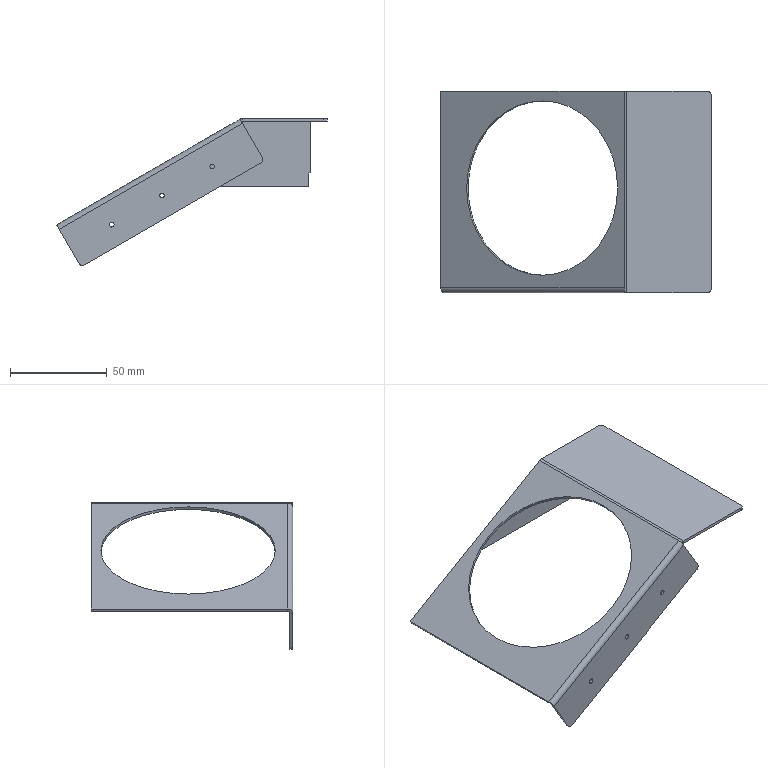Part | SolidWorks | features Cut 2, EdgeFlange 2, Fillet 1, FlatPattern 1, HoleWzd 1, ICE 1, SMBaseFlange 1, SheetMetal 1 | 1 solid | 38 faces | box 139.665 x 104 x 75.919 mm | volume 19261 mm3 | plane 22 | cylinder 16 | commonest cylinder face diameters 2.5 x6 4 x4 2 x2 5 x2 90 x2
STEP:
#1=CARTESIAN_POINT('',(-35.843,-50.5,-23.542));
#2=VERTEX_POINT('',#1);
#3=CARTESIAN_POINT('',(-35.843,-50.5,-26.042));
#4=VERTEX_POINT('',#3);
#5=CARTESIAN_POINT('',(-35.843,-50.5,-24.792));
#6=DIRECTION('',(0.,-1.,0.));
#7=DIRECTION('',(0.,0.,-1.));
#8=AXIS2_PLACEMENT_3D('',#5,#6,#7);
#9=CIRCLE('',#8,1.25);
#10=EDGE_CURVE('',#2,#4,#9,.T.);
#11=ORIENTED_EDGE('',*,*,#10,.F.);
#12=CARTESIAN_POINT('',(-35.843,-52.,-23.542));
#13=VERTEX_POINT('',#12);
#14=CARTESIAN_POINT('',(-35.843,-52.,-23.542));
#15=DIRECTION('',(0.,-1.,0.));
#16=VECTOR('',#15,1000.);
#17=LINE('',#14,#16);
#18=EDGE_CURVE('',#2,#13,#17,.T.);
#19=ORIENTED_EDGE('',*,*,#18,.T.);
#20=CARTESIAN_POINT('',(-35.843,-52.,-26.042));
#21=VERTEX_POINT('',#20);
#22=CARTESIAN_POINT('',(-35.843,-52.,-24.792));
#23=DIRECTION('',(0.,-1.,0.));
#24=DIRECTION('',(0.,0.,-1.));
#25=AXIS2_PLACEMENT_3D('',#22,#23,#24);
#26=CIRCLE('',#25,1.25);
#27=EDGE_CURVE('',#13,#21,#26,.T.);
#28=ORIENTED_EDGE('',*,*,#27,.T.);
#29=CARTESIAN_POINT('',(-35.843,-52.,-26.042));
#30=DIRECTION('',(0.,-1.,0.));
#31=VECTOR('',#30,1000.);
#32=LINE('',#29,#31);
#33=EDGE_CURVE('',#4,#21,#32,.T.);
#34=ORIENTED_EDGE('',*,*,#33,.F.);
#35=EDGE_LOOP('',(#11,#19,#28,#34));
#36=FACE_OUTER_BOUND('',#35,.T.);
#37=CARTESIAN_POINT('',(-35.843,-52.,-24.792));
#38=DIRECTION('',(0.,-1.,0.));
#39=DIRECTION('',(0.,0.,-1.));
#40=AXIS2_PLACEMENT_3D('',#37,#38,#39);
#41=CYLINDRICAL_SURFACE('',#40,1.25);
#42=ADVANCED_FACE('',(#36),#41,.F.);
#43=CARTESIAN_POINT('',(-61.823,-50.5,-38.542));
#44=VERTEX_POINT('',#43);
#45=CARTESIAN_POINT('',(-61.823,-50.5,-41.042));
#46=VERTEX_POINT('',#45);
#47=CARTESIAN_POINT('',(-61.823,-50.5,-39.792));
#48=DIRECTION('',(0.,-1.,0.));
#49=DIRECTION('',(0.,0.,-1.));
#50=AXIS2_PLACEMENT_3D('',#47,#48,#49);
#51=CIRCLE('',#50,1.25);
#52=EDGE_CURVE('',#44,#46,#51,.T.);
#53=ORIENTED_EDGE('',*,*,#52,.F.);
#54=CARTESIAN_POINT('',(-61.823,-52.,-38.542));
#55=VERTEX_POINT('',#54);
#56=CARTESIAN_POINT('',(-61.823,-52.,-38.542));
#57=DIRECTION('',(0.,-1.,0.));
#58=VECTOR('',#57,1000.);
#59=LINE('',#56,#58);
#60=EDGE_CURVE('',#44,#55,#59,.T.);
#61=ORIENTED_EDGE('',*,*,#60,.T.);
#62=CARTESIAN_POINT('',(-61.823,-52.,-41.042));
#63=VERTEX_POINT('',#62);
#64=CARTESIAN_POINT('',(-61.823,-52.,-39.792));
#65=DIRECTION('',(0.,-1.,0.));
#66=DIRECTION('',(0.,0.,-1.));
#67=AXIS2_PLACEMENT_3D('',#64,#65,#66);
#68=CIRCLE('',#67,1.25);
#69=EDGE_CURVE('',#55,#63,#68,.T.);
#70=ORIENTED_EDGE('',*,*,#69,.T.);
#71=CARTESIAN_POINT('',(-61.823,-52.,-41.042));
#72=DIRECTION('',(0.,-1.,0.));
#73=VECTOR('',#72,1000.);
#74=LINE('',#71,#73);
#75=EDGE_CURVE('',#46,#63,#74,.T.);
#76=ORIENTED_EDGE('',*,*,#75,.F.);
#77=EDGE_LOOP('',(#53,#61,#70,#76));
#78=FACE_OUTER_BOUND('',#77,.T.);
#79=CARTESIAN_POINT('',(-61.823,-52.,-39.792));
#80=DIRECTION('',(0.,-1.,0.));
#81=DIRECTION('',(0.,0.,-1.));
#82=AXIS2_PLACEMENT_3D('',#79,#80,#81);
#83=CYLINDRICAL_SURFACE('',#82,1.25);
#84=ADVANCED_FACE('',(#78),#83,.F.);
#85=CARTESIAN_POINT('',(-87.804,-50.5,-53.542));
#86=VERTEX_POINT('',#85);
#87=CARTESIAN_POINT('',(-87.804,-50.5,-56.042));
#88=VERTEX_POINT('',#87);
#89=CARTESIAN_POINT('',(-87.804,-50.5,-54.792));
#90=DIRECTION('',(0.,-1.,0.));
#91=DIRECTION('',(0.,0.,-1.));
#92=AXIS2_PLACEMENT_3D('',#89,#90,#91);
#93=CIRCLE('',#92,1.25);
#94=EDGE_CURVE('',#86,#88,#93,.T.);
#95=ORIENTED_EDGE('',*,*,#94,.F.);
#96=CARTESIAN_POINT('',(-87.804,-52.,-53.542));
#97=VERTEX_POINT('',#96);
#98=CARTESIAN_POINT('',(-87.804,-52.,-53.542));
#99=DIRECTION('',(0.,-1.,0.));
#100=VECTOR('',#99,1000.);
#101=LINE('',#98,#100);
#102=EDGE_CURVE('',#86,#97,#101,.T.);
#103=ORIENTED_EDGE('',*,*,#102,.T.);
#104=CARTESIAN_POINT('',(-87.804,-52.,-56.042));
#105=VERTEX_POINT('',#104);
#106=CARTESIAN_POINT('',(-87.804,-52.,-54.792));
#107=DIRECTION('',(0.,-1.,0.));
#108=DIRECTION('',(0.,0.,-1.));
#109=AXIS2_PLACEMENT_3D('',#106,#107,#108);
#110=CIRCLE('',#109,1.25);
#111=EDGE_CURVE('',#97,#105,#110,.T.);
#112=ORIENTED_EDGE('',*,*,#111,.T.);
#113=CARTESIAN_POINT('',(-87.804,-52.,-56.042));
#114=DIRECTION('',(0.,-1.,0.));
#115=VECTOR('',#114,1000.);
#116=LINE('',#113,#115);
#117=EDGE_CURVE('',#88,#105,#116,.T.);
#118=ORIENTED_EDGE('',*,*,#117,.F.);
#119=EDGE_LOOP('',(#95,#103,#112,#118));
#120=FACE_OUTER_BOUND('',#119,.T.);
#121=CARTESIAN_POINT('',(-87.804,-52.,-54.792));
#122=DIRECTION('',(0.,-1.,0.));
#123=DIRECTION('',(0.,0.,-1.));
#124=AXIS2_PLACEMENT_3D('',#121,#122,#123);
#125=CYLINDRICAL_SURFACE('',#124,1.25);
#126=ADVANCED_FACE('',(#120),#125,.F.);
#127=CARTESIAN_POINT('',(-102.041,2.,-48.578));
#128=VERTEX_POINT('',#127);
#129=CARTESIAN_POINT('',(-24.099,2.,-3.578));
#130=VERTEX_POINT('',#129);
#131=CARTESIAN_POINT('',(-63.07,2.,-26.078));
#132=DIRECTION('',(-0.5,0.,0.866));
#133=DIRECTION('',(0.866,0.,0.5));
#134=AXIS2_PLACEMENT_3D('',#131,#132,#133);
#135=CIRCLE('',#134,45.);
#136=EDGE_CURVE('',#128,#130,#135,.T.);
#137=ORIENTED_EDGE('',*,*,#136,.F.);
#138=CARTESIAN_POINT('',(-102.791,2.,-47.279));
#139=VERTEX_POINT('',#138);
#140=CARTESIAN_POINT('',(-97.791,2.,-55.939));
#141=DIRECTION('',(-0.5,0.,0.866));
#142=VECTOR('',#141,1000.);
#143=LINE('',#140,#142);
#144=EDGE_CURVE('',#128,#139,#143,.T.);
#145=ORIENTED_EDGE('',*,*,#144,.T.);
#146=CARTESIAN_POINT('',(-24.849,2.,-2.279));
#147=VERTEX_POINT('',#146);
#148=CARTESIAN_POINT('',(-63.82,2.,-24.779));
#149=DIRECTION('',(-0.5,0.,0.866));
#150=DIRECTION('',(0.866,0.,0.5));
#151=AXIS2_PLACEMENT_3D('',#148,#149,#150);
#152=CIRCLE('',#151,45.);
#153=EDGE_CURVE('',#139,#147,#152,.T.);
#154=ORIENTED_EDGE('',*,*,#153,.T.);
#155=CARTESIAN_POINT('',(-19.849,2.,-10.939));
#156=DIRECTION('',(-0.5,0.,0.866));
#157=VECTOR('',#156,1000.);
#158=LINE('',#155,#157);
#159=EDGE_CURVE('',#130,#147,#158,.T.);
#160=ORIENTED_EDGE('',*,*,#159,.F.);
#161=EDGE_LOOP('',(#137,#145,#154,#160));
#162=FACE_OUTER_BOUND('',#161,.T.);
#163=CARTESIAN_POINT('',(-58.82,2.,-33.439));
#164=DIRECTION('',(-0.5,0.,0.866));
#165=DIRECTION('',(0.866,0.,0.5));
#166=AXIS2_PLACEMENT_3D('',#163,#164,#165);
#167=CYLINDRICAL_SURFACE('',#166,45.);
#168=ADVANCED_FACE('',(#162),#167,.F.);
#169=CARTESIAN_POINT('',(-20.732,51.5,-1.634));
#170=VERTEX_POINT('',#169);
#171=CARTESIAN_POINT('',(-20.232,51.5,-1.5));
#172=VERTEX_POINT('',#171);
#173=CARTESIAN_POINT('',(-20.232,51.5,-2.5));
#174=DIRECTION('',(0.,1.,0.));
#175=DIRECTION('',(0.,0.,1.));
#176=AXIS2_PLACEMENT_3D('',#173,#174,#175);
#177=CIRCLE('',#176,1.);
#178=EDGE_CURVE('',#170,#172,#177,.T.);
#179=ORIENTED_EDGE('',*,*,#178,.T.);
#180=CARTESIAN_POINT('',(-20.232,-52.,-1.5));
#181=VERTEX_POINT('',#180);
#182=CARTESIAN_POINT('',(-20.232,52.,-1.5));
#183=DIRECTION('',(0.,-1.,0.));
#184=VECTOR('',#183,1000.);
#185=LINE('',#182,#184);
#186=EDGE_CURVE('',#172,#181,#185,.T.);
#187=ORIENTED_EDGE('',*,*,#186,.T.);
#188=CARTESIAN_POINT('',(-20.732,-52.,-1.634));
#189=VERTEX_POINT('',#188);
#190=CARTESIAN_POINT('',(-20.232,-52.,-2.5));
#191=DIRECTION('',(0.,-1.,0.));
#192=DIRECTION('',(0.,0.,1.));
#193=AXIS2_PLACEMENT_3D('',#190,#191,#192);
#194=CIRCLE('',#193,1.);
#195=EDGE_CURVE('',#181,#189,#194,.T.);
#196=ORIENTED_EDGE('',*,*,#195,.T.);
#197=CARTESIAN_POINT('',(-20.732,-51.791,-1.634));
#198=VERTEX_POINT('',#197);
#199=CARTESIAN_POINT('',(-20.732,-52.,-1.634));
#200=DIRECTION('',(0.,1.,0.));
#201=VECTOR('',#200,1000.);
#202=LINE('',#199,#201);
#203=EDGE_CURVE('',#189,#198,#202,.T.);
#204=ORIENTED_EDGE('',*,*,#203,.T.);
#205=CARTESIAN_POINT('',(-20.732,-49.5,-1.634));
#206=VERTEX_POINT('',#205);
#207=CARTESIAN_POINT('',(-20.732,-52.,-1.634));
#208=DIRECTION('',(0.,1.,0.));
#209=VECTOR('',#208,1000.);
#210=LINE('',#207,#209);
#211=EDGE_CURVE('',#198,#206,#210,.T.);
#212=ORIENTED_EDGE('',*,*,#211,.T.);
#213=CARTESIAN_POINT('',(-20.732,-52.,-1.634));
#214=DIRECTION('',(0.,1.,0.));
#215=VECTOR('',#214,1000.);
#216=LINE('',#213,#215);
#217=EDGE_CURVE('',#206,#170,#216,.T.);
#218=ORIENTED_EDGE('',*,*,#217,.T.);
#219=EDGE_LOOP('',(#179,#187,#196,#204,#212,#218));
#220=FACE_OUTER_BOUND('',#219,.T.);
#221=CARTESIAN_POINT('',(-20.232,52.,-2.5));
#222=DIRECTION('',(0.,1.,0.));
#223=DIRECTION('',(-0.5,0.,0.866));
#224=AXIS2_PLACEMENT_3D('',#221,#222,#223);
#225=CYLINDRICAL_SURFACE('',#224,1.);
#226=ADVANCED_FACE('',(#220),#225,.F.);
#227=CARTESIAN_POINT('',(-21.482,-52.,-0.3349));
#228=VERTEX_POINT('',#227);
#229=CARTESIAN_POINT('',(-21.482,-49.5,-0.3349));
#230=VERTEX_POINT('',#229);
#231=CARTESIAN_POINT('',(-21.482,0.,-0.3349));
#232=DIRECTION('',(0.,1.,0.));
#233=VECTOR('',#232,1000.);
#234=LINE('',#231,#233);
#235=EDGE_CURVE('',#228,#230,#234,.T.);
#236=ORIENTED_EDGE('',*,*,#235,.T.);
#237=CARTESIAN_POINT('',(-20.232,-49.5,-2.5));
#238=DIRECTION('',(0.866,0.,0.5));
#239=DIRECTION('',(-0.5,0.,0.866));
#240=AXIS2_PLACEMENT_3D('',#237,#238,#239);
#241=CIRCLE('',#240,2.5);
#242=EDGE_CURVE('',#230,#198,#241,.T.);
#243=ORIENTED_EDGE('',*,*,#242,.T.);
#244=ORIENTED_EDGE('',*,*,#203,.F.);
#245=CARTESIAN_POINT('',(-21.482,-52.,-0.3349));
#246=DIRECTION('',(-0.5,0.,0.866));
#247=VECTOR('',#246,1000.);
#248=LINE('',#245,#247);
#249=EDGE_CURVE('',#189,#228,#248,.T.);
#250=ORIENTED_EDGE('',*,*,#249,.T.);
#251=EDGE_LOOP('',(#236,#243,#244,#250));
#252=FACE_OUTER_BOUND('',#251,.T.);
#253=CARTESIAN_POINT('',(-20.732,-49.5,-1.634));
#254=DIRECTION('',(-0.866,0.,-0.5));
#255=DIRECTION('',(-0.5,0.,0.866));
#256=AXIS2_PLACEMENT_3D('',#253,#254,#255);
#257=PLANE('',#256);
#258=ADVANCED_FACE('',(#252),#257,.T.);
#259=CARTESIAN_POINT('',(-63.82,2.,-24.779));
#260=DIRECTION('',(-0.5,0.,0.866));
#261=DIRECTION('',(0.866,0.,0.5));
#262=AXIS2_PLACEMENT_3D('',#259,#260,#261);
#263=CIRCLE('',#262,45.);
#264=EDGE_CURVE('',#147,#139,#263,.T.);
#265=ORIENTED_EDGE('',*,*,#264,.F.);
#266=ORIENTED_EDGE('',*,*,#153,.F.);
#267=EDGE_LOOP('',(#265,#266));
#268=FACE_BOUND('',#267,.T.);
#269=CARTESIAN_POINT('',(-116.165,-49.5,-55.));
#270=VERTEX_POINT('',#269);
#271=CARTESIAN_POINT('',(-116.165,52.,-55.));
#272=VERTEX_POINT('',#271);
#273=CARTESIAN_POINT('',(-116.165,52.,-55.));
#274=DIRECTION('',(0.,1.,0.));
#275=VECTOR('',#274,1000.);
#276=LINE('',#273,#275);
#277=EDGE_CURVE('',#270,#272,#276,.T.);
#278=ORIENTED_EDGE('',*,*,#277,.F.);
#279=CARTESIAN_POINT('',(-116.165,-49.5,-55.));
#280=DIRECTION('',(0.866,0.,0.5));
#281=VECTOR('',#280,1000.);
#282=LINE('',#279,#281);
#283=EDGE_CURVE('',#270,#230,#282,.T.);
#284=ORIENTED_EDGE('',*,*,#283,.T.);
#285=CARTESIAN_POINT('',(-21.482,52.,-0.3349));
#286=VERTEX_POINT('',#285);
#287=CARTESIAN_POINT('',(-21.482,0.,-0.3349));
#288=DIRECTION('',(0.,1.,0.));
#289=VECTOR('',#288,1000.);
#290=LINE('',#287,#289);
#291=EDGE_CURVE('',#230,#286,#290,.T.);
#292=ORIENTED_EDGE('',*,*,#291,.T.);
#293=CARTESIAN_POINT('',(-21.25,52.,-0.201));
#294=DIRECTION('',(0.866,0.,0.5));
#295=VECTOR('',#294,1000.);
#296=LINE('',#293,#295);
#297=EDGE_CURVE('',#272,#286,#296,.T.);
#298=ORIENTED_EDGE('',*,*,#297,.F.);
#299=EDGE_LOOP('',(#278,#284,#292,#298));
#300=FACE_OUTER_BOUND('',#299,.T.);
#301=CARTESIAN_POINT('',(-2.975,0.,10.35));
#302=DIRECTION('',(-0.5,0.,0.866));
#303=DIRECTION('',(0.866,0.,0.5));
#304=AXIS2_PLACEMENT_3D('',#301,#302,#303);
#305=PLANE('',#304);
#306=ADVANCED_FACE('',(#268,#300),#305,.T.);
#307=CARTESIAN_POINT('',(-63.07,2.,-26.078));
#308=DIRECTION('',(-0.5,0.,0.866));
#309=DIRECTION('',(0.866,0.,0.5));
#310=AXIS2_PLACEMENT_3D('',#307,#308,#309);
#311=CIRCLE('',#310,45.);
#312=EDGE_CURVE('',#130,#128,#311,.T.);
#313=ORIENTED_EDGE('',*,*,#312,.T.);
#314=ORIENTED_EDGE('',*,*,#136,.T.);
#315=EDGE_LOOP('',(#313,#314));
#316=FACE_BOUND('',#315,.T.);
#317=CARTESIAN_POINT('',(-115.415,52.,-56.299));
#318=VERTEX_POINT('',#317);
#319=CARTESIAN_POINT('',(-78.756,52.,-35.134));
#320=VERTEX_POINT('',#319);
#321=CARTESIAN_POINT('',(-2.225,52.,9.051));
#322=DIRECTION('',(0.866,0.,0.5));
#323=VECTOR('',#322,1000.);
#324=LINE('',#321,#323);
#325=EDGE_CURVE('',#318,#320,#324,.T.);
#326=ORIENTED_EDGE('',*,*,#325,.T.);
#327=CARTESIAN_POINT('',(-78.756,51.5,-35.134));
#328=VERTEX_POINT('',#327);
#329=CARTESIAN_POINT('',(-78.756,51.5,-35.134));
#330=DIRECTION('',(0.,1.,0.));
#331=VECTOR('',#330,1000.);
#332=LINE('',#329,#331);
#333=EDGE_CURVE('',#328,#320,#332,.T.);
#334=ORIENTED_EDGE('',*,*,#333,.F.);
#335=CARTESIAN_POINT('',(-20.732,51.5,-1.634));
#336=DIRECTION('',(0.866,0.,0.5));
#337=VECTOR('',#336,1000.);
#338=LINE('',#335,#337);
#339=EDGE_CURVE('',#328,#170,#338,.T.);
#340=ORIENTED_EDGE('',*,*,#339,.T.);
#341=ORIENTED_EDGE('',*,*,#217,.F.);
#342=CARTESIAN_POINT('',(-115.415,-49.5,-56.299));
#343=VERTEX_POINT('',#342);
#344=CARTESIAN_POINT('',(-115.415,-49.5,-56.299));
#345=DIRECTION('',(0.866,0.,0.5));
#346=VECTOR('',#345,1000.);
#347=LINE('',#344,#346);
#348=EDGE_CURVE('',#343,#206,#347,.T.);
#349=ORIENTED_EDGE('',*,*,#348,.F.);
#350=CARTESIAN_POINT('',(-115.415,0.,-56.299));
#351=DIRECTION('',(0.,1.,0.));
#352=VECTOR('',#351,1000.);
#353=LINE('',#350,#352);
#354=EDGE_CURVE('',#343,#318,#353,.T.);
#355=ORIENTED_EDGE('',*,*,#354,.T.);
#356=EDGE_LOOP('',(#326,#334,#340,#341,#349,#355));
#357=FACE_OUTER_BOUND('',#356,.T.);
#358=CARTESIAN_POINT('',(-2.225,0.,9.051));
#359=DIRECTION('',(-0.5,0.,0.866));
#360=DIRECTION('',(0.866,0.,0.5));
#361=AXIS2_PLACEMENT_3D('',#358,#359,#360);
#362=PLANE('',#361);
#363=ADVANCED_FACE('',(#316,#357),#362,.F.);
#364=ORIENTED_EDGE('',*,*,#354,.F.);
#365=CARTESIAN_POINT('',(-115.415,-49.5,-56.299));
#366=DIRECTION('',(-0.5,0.,0.866));
#367=VECTOR('',#366,1000.);
#368=LINE('',#365,#367);
#369=EDGE_CURVE('',#343,#270,#368,.T.);
#370=ORIENTED_EDGE('',*,*,#369,.T.);
#371=ORIENTED_EDGE('',*,*,#277,.T.);
#372=CARTESIAN_POINT('',(-116.165,52.,-55.));
#373=DIRECTION('',(0.5,0.,-0.866));
#374=VECTOR('',#373,1000.);
#375=LINE('',#372,#374);
#376=EDGE_CURVE('',#272,#318,#375,.T.);
#377=ORIENTED_EDGE('',*,*,#376,.T.);
#378=EDGE_LOOP('',(#364,#370,#371,#377));
#379=FACE_OUTER_BOUND('',#378,.T.);
#380=CARTESIAN_POINT('',(-116.165,52.,-55.));
#381=DIRECTION('',(-0.866,0.,-0.5));
#382=DIRECTION('',(-0.5,0.,0.866));
#383=AXIS2_PLACEMENT_3D('',#380,#381,#382);
#384=PLANE('',#383);
#385=ADVANCED_FACE('',(#379),#384,.T.);
#386=CARTESIAN_POINT('',(-20.232,52.,0.));
#387=VERTEX_POINT('',#386);
#388=CARTESIAN_POINT('',(-20.232,52.,-2.5));
#389=DIRECTION('',(0.,1.,0.));
#390=DIRECTION('',(0.,0.,1.));
#391=AXIS2_PLACEMENT_3D('',#388,#389,#390);
#392=CIRCLE('',#391,2.5);
#393=EDGE_CURVE('',#286,#387,#392,.T.);
#394=ORIENTED_EDGE('',*,*,#393,.T.);
#395=CARTESIAN_POINT('',(21.5,52.,0.));
#396=VERTEX_POINT('',#395);
#397=CARTESIAN_POINT('',(-23.5,52.,0.));
#398=DIRECTION('',(-1.,0.,0.));
#399=VECTOR('',#398,1000.);
#400=LINE('',#397,#399);
#401=EDGE_CURVE('',#396,#387,#400,.T.);
#402=ORIENTED_EDGE('',*,*,#401,.F.);
#403=CARTESIAN_POINT('',(21.5,52.,-1.5));
#404=VERTEX_POINT('',#403);
#405=CARTESIAN_POINT('',(21.5,52.,-1.5));
#406=DIRECTION('',(0.,0.,-1.));
#407=VECTOR('',#406,1000.);
#408=LINE('',#405,#407);
#409=EDGE_CURVE('',#396,#404,#408,.T.);
#410=ORIENTED_EDGE('',*,*,#409,.T.);
#411=CARTESIAN_POINT('',(14.768,52.,-1.5));
#412=VERTEX_POINT('',#411);
#413=CARTESIAN_POINT('',(-23.5,52.,-1.5));
#414=DIRECTION('',(-1.,0.,0.));
#415=VECTOR('',#414,1000.);
#416=LINE('',#413,#415);
#417=EDGE_CURVE('',#404,#412,#416,.T.);
#418=ORIENTED_EDGE('',*,*,#417,.T.);
#419=CARTESIAN_POINT('',(14.768,52.,-28.134));
#420=VERTEX_POINT('',#419);
#421=CARTESIAN_POINT('',(14.768,52.,-1.5));
#422=DIRECTION('',(0.,0.,-1.));
#423=VECTOR('',#422,1000.);
#424=LINE('',#421,#423);
#425=EDGE_CURVE('',#412,#420,#424,.T.);
#426=ORIENTED_EDGE('',*,*,#425,.T.);
#427=CARTESIAN_POINT('',(13.843,52.,-28.134));
#428=VERTEX_POINT('',#427);
#429=CARTESIAN_POINT('',(14.768,52.,-28.134));
#430=DIRECTION('',(1.,0.,0.));
#431=VECTOR('',#430,1000.);
#432=LINE('',#429,#431);
#433=EDGE_CURVE('',#428,#420,#432,.T.);
#434=ORIENTED_EDGE('',*,*,#433,.F.);
#435=CARTESIAN_POINT('',(13.843,52.,-35.134));
#436=VERTEX_POINT('',#435);
#437=CARTESIAN_POINT('',(13.843,52.,-35.134));
#438=DIRECTION('',(0.,0.,1.));
#439=VECTOR('',#438,1000.);
#440=LINE('',#437,#439);
#441=EDGE_CURVE('',#436,#428,#440,.T.);
#442=ORIENTED_EDGE('',*,*,#441,.F.);
#443=CARTESIAN_POINT('',(14.768,52.,-35.134));
#444=DIRECTION('',(-1.,0.,0.));
#445=VECTOR('',#444,1000.);
#446=LINE('',#443,#445);
#447=EDGE_CURVE('',#436,#320,#446,.T.);
#448=ORIENTED_EDGE('',*,*,#447,.T.);
#449=ORIENTED_EDGE('',*,*,#325,.F.);
#450=ORIENTED_EDGE('',*,*,#376,.F.);
#451=ORIENTED_EDGE('',*,*,#297,.T.);
#452=EDGE_LOOP('',(#394,#402,#410,#418,#426,#434,#442,#448,#449,#450,#451));
#453=FACE_OUTER_BOUND('',#452,.T.);
#454=CARTESIAN_POINT('',(-23.5,52.,-1.5));
#455=DIRECTION('',(0.,1.,0.));
#456=DIRECTION('',(0.,0.,1.));
#457=AXIS2_PLACEMENT_3D('',#454,#455,#456);
#458=PLANE('',#457);
#459=ADVANCED_FACE('',(#453),#458,.T.);
#460=CARTESIAN_POINT('',(14.768,51.5,-1.5));
#461=VERTEX_POINT('',#460);
#462=CARTESIAN_POINT('',(-20.232,51.5,-1.5));
#463=DIRECTION('',(1.,0.,0.));
#464=VECTOR('',#463,1000.);
#465=LINE('',#462,#464);
#466=EDGE_CURVE('',#172,#461,#465,.T.);
#467=ORIENTED_EDGE('',*,*,#466,.T.);
#468=CARTESIAN_POINT('',(14.768,51.5,-1.5));
#469=DIRECTION('',(0.,1.,0.));
#470=VECTOR('',#469,1000.);
#471=LINE('',#468,#470);
#472=EDGE_CURVE('',#461,#412,#471,.T.);
#473=ORIENTED_EDGE('',*,*,#472,.T.);
#474=ORIENTED_EDGE('',*,*,#417,.F.);
#475=CARTESIAN_POINT('',(23.5,50.,-1.5));
#476=VERTEX_POINT('',#475);
#477=CARTESIAN_POINT('',(21.5,50.,-1.5));
#478=DIRECTION('',(0.,0.,-1.));
#479=DIRECTION('',(1.,0.,0.));
#480=AXIS2_PLACEMENT_3D('',#477,#478,#479);
#481=CIRCLE('',#480,2.);
#482=EDGE_CURVE('',#404,#476,#481,.T.);
#483=ORIENTED_EDGE('',*,*,#482,.T.);
#484=CARTESIAN_POINT('',(23.5,-50.,-1.5));
#485=VERTEX_POINT('',#484);
#486=CARTESIAN_POINT('',(23.5,52.,-1.5));
#487=DIRECTION('',(0.,1.,0.));
#488=VECTOR('',#487,1000.);
#489=LINE('',#486,#488);
#490=EDGE_CURVE('',#485,#476,#489,.T.);
#491=ORIENTED_EDGE('',*,*,#490,.F.);
#492=CARTESIAN_POINT('',(21.5,-52.,-1.5));
#493=VERTEX_POINT('',#492);
#494=CARTESIAN_POINT('',(21.5,-50.,-1.5));
#495=DIRECTION('',(0.,0.,-1.));
#496=DIRECTION('',(1.,0.,0.));
#497=AXIS2_PLACEMENT_3D('',#494,#495,#496);
#498=CIRCLE('',#497,2.);
#499=EDGE_CURVE('',#485,#493,#498,.T.);
#500=ORIENTED_EDGE('',*,*,#499,.T.);
#501=CARTESIAN_POINT('',(-23.5,-52.,-1.5));
#502=DIRECTION('',(1.,0.,0.));
#503=VECTOR('',#502,1000.);
#504=LINE('',#501,#503);
#505=EDGE_CURVE('',#181,#493,#504,.T.);
#506=ORIENTED_EDGE('',*,*,#505,.F.);
#507=ORIENTED_EDGE('',*,*,#186,.F.);
#508=EDGE_LOOP('',(#467,#473,#474,#483,#491,#500,#506,#507));
#509=FACE_OUTER_BOUND('',#508,.T.);
#510=CARTESIAN_POINT('',(0.,0.,-1.5));
#511=DIRECTION('',(0.,0.,1.));
#512=DIRECTION('',(1.,0.,0.));
#513=AXIS2_PLACEMENT_3D('',#510,#511,#512);
#514=PLANE('',#513);
#515=ADVANCED_FACE('',(#509),#514,.F.);
#516=CARTESIAN_POINT('',(23.5,-50.,0.));
#517=VERTEX_POINT('',#516);
#518=CARTESIAN_POINT('',(23.5,50.,0.));
#519=VERTEX_POINT('',#518);
#520=CARTESIAN_POINT('',(23.5,52.,0.));
#521=DIRECTION('',(0.,1.,0.));
#522=VECTOR('',#521,1000.);
#523=LINE('',#520,#522);
#524=EDGE_CURVE('',#517,#519,#523,.T.);
#525=ORIENTED_EDGE('',*,*,#524,.T.);
#526=CARTESIAN_POINT('',(21.5,50.,0.));
#527=DIRECTION('',(0.,0.,1.));
#528=DIRECTION('',(1.,0.,0.));
#529=AXIS2_PLACEMENT_3D('',#526,#527,#528);
#530=CIRCLE('',#529,2.);
#531=EDGE_CURVE('',#519,#396,#530,.T.);
#532=ORIENTED_EDGE('',*,*,#531,.T.);
#533=ORIENTED_EDGE('',*,*,#401,.T.);
#534=CARTESIAN_POINT('',(-20.232,-52.,0.));
#535=VERTEX_POINT('',#534);
#536=CARTESIAN_POINT('',(-20.232,52.,0.));
#537=DIRECTION('',(0.,-1.,0.));
#538=VECTOR('',#537,1000.);
#539=LINE('',#536,#538);
#540=EDGE_CURVE('',#387,#535,#539,.T.);
#541=ORIENTED_EDGE('',*,*,#540,.T.);
#542=CARTESIAN_POINT('',(21.5,-52.,0.));
#543=VERTEX_POINT('',#542);
#544=CARTESIAN_POINT('',(-23.5,-52.,0.));
#545=DIRECTION('',(1.,0.,0.));
#546=VECTOR('',#545,1000.);
#547=LINE('',#544,#546);
#548=EDGE_CURVE('',#535,#543,#547,.T.);
#549=ORIENTED_EDGE('',*,*,#548,.T.);
#550=CARTESIAN_POINT('',(21.5,-50.,0.));
#551=DIRECTION('',(0.,0.,1.));
#552=DIRECTION('',(1.,0.,0.));
#553=AXIS2_PLACEMENT_3D('',#550,#551,#552);
#554=CIRCLE('',#553,2.);
#555=EDGE_CURVE('',#543,#517,#554,.T.);
#556=ORIENTED_EDGE('',*,*,#555,.T.);
#557=EDGE_LOOP('',(#525,#532,#533,#541,#549,#556));
#558=FACE_OUTER_BOUND('',#557,.T.);
#559=CARTESIAN_POINT('',(0.,0.,0.));
#560=DIRECTION('',(0.,0.,1.));
#561=DIRECTION('',(1.,0.,0.));
#562=AXIS2_PLACEMENT_3D('',#559,#560,#561);
#563=PLANE('',#562);
#564=ADVANCED_FACE('',(#558),#563,.T.);
#565=ORIENTED_EDGE('',*,*,#490,.T.);
#566=CARTESIAN_POINT('',(23.5,50.,-1.5));
#567=DIRECTION('',(0.,0.,1.));
#568=VECTOR('',#567,1000.);
#569=LINE('',#566,#568);
#570=EDGE_CURVE('',#476,#519,#569,.T.);
#571=ORIENTED_EDGE('',*,*,#570,.T.);
#572=ORIENTED_EDGE('',*,*,#524,.F.);
#573=CARTESIAN_POINT('',(23.5,-50.,-1.5));
#574=DIRECTION('',(0.,0.,-1.));
#575=VECTOR('',#574,1000.);
#576=LINE('',#573,#575);
#577=EDGE_CURVE('',#517,#485,#576,.T.);
#578=ORIENTED_EDGE('',*,*,#577,.T.);
#579=EDGE_LOOP('',(#565,#571,#572,#578));
#580=FACE_OUTER_BOUND('',#579,.T.);
#581=CARTESIAN_POINT('',(23.5,52.,-1.5));
#582=DIRECTION('',(1.,0.,0.));
#583=DIRECTION('',(0.,1.,0.));
#584=AXIS2_PLACEMENT_3D('',#581,#582,#583);
#585=PLANE('',#584);
#586=ADVANCED_FACE('',(#580),#585,.T.);
#587=ORIENTED_EDGE('',*,*,#505,.T.);
#588=CARTESIAN_POINT('',(21.5,-52.,-1.5));
#589=DIRECTION('',(0.,0.,1.));
#590=VECTOR('',#589,1000.);
#591=LINE('',#588,#590);
#592=EDGE_CURVE('',#493,#543,#591,.T.);
#593=ORIENTED_EDGE('',*,*,#592,.T.);
#594=ORIENTED_EDGE('',*,*,#548,.F.);
#595=CARTESIAN_POINT('',(-20.232,-52.,-1.5));
#596=DIRECTION('',(0.,0.,1.));
#597=VECTOR('',#596,1000.);
#598=LINE('',#595,#597);
#599=EDGE_CURVE('',#181,#535,#598,.T.);
#600=ORIENTED_EDGE('',*,*,#599,.F.);
#601=EDGE_LOOP('',(#587,#593,#594,#600));
#602=FACE_OUTER_BOUND('',#601,.T.);
#603=CARTESIAN_POINT('',(-23.5,-52.,-1.5));
#604=DIRECTION('',(0.,-1.,0.));
#605=DIRECTION('',(0.,0.,-1.));
#606=AXIS2_PLACEMENT_3D('',#603,#604,#605);
#607=PLANE('',#606);
#608=ADVANCED_FACE('',(#602),#607,.T.);
#609=ORIENTED_EDGE('',*,*,#249,.F.);
#610=ORIENTED_EDGE('',*,*,#195,.F.);
#611=ORIENTED_EDGE('',*,*,#599,.T.);
#612=CARTESIAN_POINT('',(-20.232,-52.,-2.5));
#613=DIRECTION('',(0.,-1.,0.));
#614=DIRECTION('',(0.,0.,1.));
#615=AXIS2_PLACEMENT_3D('',#612,#613,#614);
#616=CIRCLE('',#615,2.5);
#617=EDGE_CURVE('',#535,#228,#616,.T.);
#618=ORIENTED_EDGE('',*,*,#617,.T.);
#619=EDGE_LOOP('',(#609,#610,#611,#618));
#620=FACE_OUTER_BOUND('',#619,.T.);
#621=CARTESIAN_POINT('',(-20.232,-52.,-2.5));
#622=DIRECTION('',(0.,-1.,0.));
#623=DIRECTION('',(0.,0.,-1.));
#624=AXIS2_PLACEMENT_3D('',#621,#622,#623);
#625=PLANE('',#624);
#626=ADVANCED_FACE('',(#620),#625,.T.);
#627=ORIENTED_EDGE('',*,*,#540,.F.);
#628=ORIENTED_EDGE('',*,*,#393,.F.);
#629=ORIENTED_EDGE('',*,*,#291,.F.);
#630=ORIENTED_EDGE('',*,*,#235,.F.);
#631=ORIENTED_EDGE('',*,*,#617,.F.);
#632=EDGE_LOOP('',(#627,#628,#629,#630,#631));
#633=FACE_OUTER_BOUND('',#632,.T.);
#634=CARTESIAN_POINT('',(-20.232,52.,-2.5));
#635=DIRECTION('',(0.,1.,0.));
#636=DIRECTION('',(-0.5,0.,0.866));
#637=AXIS2_PLACEMENT_3D('',#634,#635,#636);
#638=CYLINDRICAL_SURFACE('',#637,2.5);
#639=ADVANCED_FACE('',(#633),#638,.T.);
#640=ORIENTED_EDGE('',*,*,#211,.F.);
#641=CARTESIAN_POINT('',(-20.232,-52.,-2.5));
#642=VERTEX_POINT('',#641);
#643=CARTESIAN_POINT('',(-20.232,-49.5,-2.5));
#644=DIRECTION('',(0.866,0.,0.5));
#645=DIRECTION('',(-0.5,0.,0.866));
#646=AXIS2_PLACEMENT_3D('',#643,#644,#645);
#647=CIRCLE('',#646,2.5);
#648=EDGE_CURVE('',#198,#642,#647,.T.);
#649=ORIENTED_EDGE('',*,*,#648,.T.);
#650=CARTESIAN_POINT('',(-20.232,-50.5,-2.5));
#651=VERTEX_POINT('',#650);
#652=CARTESIAN_POINT('',(-20.232,-52.,-2.5));
#653=DIRECTION('',(0.,-1.,0.));
#654=VECTOR('',#653,1000.);
#655=LINE('',#652,#654);
#656=EDGE_CURVE('',#651,#642,#655,.T.);
#657=ORIENTED_EDGE('',*,*,#656,.F.);
#658=CARTESIAN_POINT('',(-20.232,-49.5,-2.5));
#659=DIRECTION('',(0.866,0.,0.5));
#660=DIRECTION('',(-0.5,0.,0.866));
#661=AXIS2_PLACEMENT_3D('',#658,#659,#660);
#662=CIRCLE('',#661,1.);
#663=EDGE_CURVE('',#206,#651,#662,.T.);
#664=ORIENTED_EDGE('',*,*,#663,.F.);
#665=EDGE_LOOP('',(#640,#649,#657,#664));
#666=FACE_OUTER_BOUND('',#665,.T.);
#667=CARTESIAN_POINT('',(-20.232,-49.5,-2.5));
#668=DIRECTION('',(0.866,0.,0.5));
#669=DIRECTION('',(0.5,0.,-0.866));
#670=AXIS2_PLACEMENT_3D('',#667,#668,#669);
#671=PLANE('',#670);
#672=ADVANCED_FACE('',(#666),#671,.T.);
#673=CARTESIAN_POINT('',(-114.915,-50.5,-57.165));
#674=VERTEX_POINT('',#673);
#675=CARTESIAN_POINT('',(-114.915,-49.5,-57.165));
#676=DIRECTION('',(-0.866,0.,-0.5));
#677=DIRECTION('',(-0.5,0.,0.866));
#678=AXIS2_PLACEMENT_3D('',#675,#676,#677);
#679=CIRCLE('',#678,1.);
#680=EDGE_CURVE('',#674,#343,#679,.T.);
#681=ORIENTED_EDGE('',*,*,#680,.F.);
#682=CARTESIAN_POINT('',(-114.915,-52.,-57.165));
#683=VERTEX_POINT('',#682);
#684=CARTESIAN_POINT('',(-114.915,-50.5,-57.165));
#685=DIRECTION('',(0.,-1.,0.));
#686=VECTOR('',#685,1000.);
#687=LINE('',#684,#686);
#688=EDGE_CURVE('',#674,#683,#687,.T.);
#689=ORIENTED_EDGE('',*,*,#688,.T.);
#690=CARTESIAN_POINT('',(-114.915,-49.5,-57.165));
#691=DIRECTION('',(-0.866,0.,-0.5));
#692=DIRECTION('',(-0.5,0.,0.866));
#693=AXIS2_PLACEMENT_3D('',#690,#691,#692);
#694=CIRCLE('',#693,2.5);
#695=EDGE_CURVE('',#683,#270,#694,.T.);
#696=ORIENTED_EDGE('',*,*,#695,.T.);
#697=ORIENTED_EDGE('',*,*,#369,.F.);
#698=EDGE_LOOP('',(#681,#689,#696,#697));
#699=FACE_OUTER_BOUND('',#698,.T.);
#700=CARTESIAN_POINT('',(-114.915,-49.5,-57.165));
#701=DIRECTION('',(0.866,0.,0.5));
#702=DIRECTION('',(0.5,0.,-0.866));
#703=AXIS2_PLACEMENT_3D('',#700,#701,#702);
#704=PLANE('',#703);
#705=ADVANCED_FACE('',(#699),#704,.F.);
#706=ORIENTED_EDGE('',*,*,#283,.F.);
#707=ORIENTED_EDGE('',*,*,#695,.F.);
#708=CARTESIAN_POINT('',(-3.975,-52.,6.886));
#709=DIRECTION('',(-0.866,0.,-0.5));
#710=VECTOR('',#709,1000.);
#711=LINE('',#708,#710);
#712=EDGE_CURVE('',#642,#683,#711,.T.);
#713=ORIENTED_EDGE('',*,*,#712,.F.);
#714=ORIENTED_EDGE('',*,*,#648,.F.);
#715=ORIENTED_EDGE('',*,*,#242,.F.);
#716=EDGE_LOOP('',(#706,#707,#713,#714,#715));
#717=FACE_OUTER_BOUND('',#716,.T.);
#718=CARTESIAN_POINT('',(-114.915,-49.5,-57.165));
#719=DIRECTION('',(-0.866,0.,-0.5));
#720=DIRECTION('',(0.,-1.,0.));
#721=AXIS2_PLACEMENT_3D('',#718,#719,#720);
#722=CYLINDRICAL_SURFACE('',#721,2.5);
#723=ADVANCED_FACE('',(#717),#722,.T.);
#724=ORIENTED_EDGE('',*,*,#348,.T.);
#725=ORIENTED_EDGE('',*,*,#663,.T.);
#726=CARTESIAN_POINT('',(-20.232,-50.5,-2.5));
#727=DIRECTION('',(-0.866,0.,-0.5));
#728=VECTOR('',#727,1000.);
#729=LINE('',#726,#728);
#730=EDGE_CURVE('',#651,#674,#729,.T.);
#731=ORIENTED_EDGE('',*,*,#730,.T.);
#732=ORIENTED_EDGE('',*,*,#680,.T.);
#733=EDGE_LOOP('',(#724,#725,#731,#732));
#734=FACE_OUTER_BOUND('',#733,.T.);
#735=CARTESIAN_POINT('',(-114.915,-49.5,-57.165));
#736=DIRECTION('',(-0.866,0.,-0.5));
#737=DIRECTION('',(0.,-1.,0.));
#738=AXIS2_PLACEMENT_3D('',#735,#736,#737);
#739=CYLINDRICAL_SURFACE('',#738,1.);
#740=ADVANCED_FACE('',(#734),#739,.F.);
#741=CARTESIAN_POINT('',(-104.665,-50.5,-74.919));
#742=VERTEX_POINT('',#741);
#743=CARTESIAN_POINT('',(-110.939,-50.5,-64.051));
#744=DIRECTION('',(-0.5,0.,0.866));
#745=VECTOR('',#744,1000.);
#746=LINE('',#743,#745);
#747=EDGE_CURVE('',#742,#674,#746,.T.);
#748=ORIENTED_EDGE('',*,*,#747,.F.);
#749=CARTESIAN_POINT('',(-104.665,-52.,-74.919));
#750=VERTEX_POINT('',#749);
#751=CARTESIAN_POINT('',(-104.665,-52.,-74.919));
#752=DIRECTION('',(0.,-1.,0.));
#753=VECTOR('',#752,1000.);
#754=LINE('',#751,#753);
#755=EDGE_CURVE('',#742,#750,#754,.T.);
#756=ORIENTED_EDGE('',*,*,#755,.T.);
#757=CARTESIAN_POINT('',(-115.415,-52.,-56.299));
#758=DIRECTION('',(-0.5,0.,0.866));
#759=VECTOR('',#758,1000.);
#760=LINE('',#757,#759);
#761=EDGE_CURVE('',#750,#683,#760,.T.);
#762=ORIENTED_EDGE('',*,*,#761,.T.);
#763=ORIENTED_EDGE('',*,*,#688,.F.);
#764=EDGE_LOOP('',(#748,#756,#762,#763));
#765=FACE_OUTER_BOUND('',#764,.T.);
#766=CARTESIAN_POINT('',(-115.415,-52.,-56.299));
#767=DIRECTION('',(-0.866,0.,-0.5));
#768=DIRECTION('',(-0.5,0.,0.866));
#769=AXIS2_PLACEMENT_3D('',#766,#767,#768);
#770=PLANE('',#769);
#771=ADVANCED_FACE('',(#765),#770,.T.);
#772=CARTESIAN_POINT('',(-9.982,-52.,-20.254));
#773=VERTEX_POINT('',#772);
#774=CARTESIAN_POINT('',(-8.982,-52.,-21.986));
#775=DIRECTION('',(0.5,0.,-0.866));
#776=VECTOR('',#775,1000.);
#777=LINE('',#774,#776);
#778=EDGE_CURVE('',#642,#773,#777,.T.);
#779=ORIENTED_EDGE('',*,*,#778,.T.);
#780=CARTESIAN_POINT('',(-9.982,-50.5,-20.254));
#781=VERTEX_POINT('',#780);
#782=CARTESIAN_POINT('',(-9.982,-52.,-20.254));
#783=DIRECTION('',(0.,1.,0.));
#784=VECTOR('',#783,1000.);
#785=LINE('',#782,#784);
#786=EDGE_CURVE('',#773,#781,#785,.T.);
#787=ORIENTED_EDGE('',*,*,#786,.T.);
#788=CARTESIAN_POINT('',(-16.257,-50.5,-9.386));
#789=DIRECTION('',(0.5,0.,-0.866));
#790=VECTOR('',#789,1000.);
#791=LINE('',#788,#790);
#792=EDGE_CURVE('',#651,#781,#791,.T.);
#793=ORIENTED_EDGE('',*,*,#792,.F.);
#794=ORIENTED_EDGE('',*,*,#656,.T.);
#795=EDGE_LOOP('',(#779,#787,#793,#794));
#796=FACE_OUTER_BOUND('',#795,.T.);
#797=CARTESIAN_POINT('',(-8.982,-52.,-21.986));
#798=DIRECTION('',(0.866,0.,0.5));
#799=DIRECTION('',(0.5,0.,-0.866));
#800=AXIS2_PLACEMENT_3D('',#797,#798,#799);
#801=PLANE('',#800);
#802=ADVANCED_FACE('',(#796),#801,.T.);
#803=CARTESIAN_POINT('',(-35.843,-52.,-24.792));
#804=DIRECTION('',(0.,-1.,0.));
#805=DIRECTION('',(0.,0.,-1.));
#806=AXIS2_PLACEMENT_3D('',#803,#804,#805);
#807=CIRCLE('',#806,1.25);
#808=EDGE_CURVE('',#21,#13,#807,.T.);
#809=ORIENTED_EDGE('',*,*,#808,.F.);
#810=ORIENTED_EDGE('',*,*,#27,.F.);
#811=EDGE_LOOP('',(#809,#810));
#812=FACE_BOUND('',#811,.T.);
#813=CARTESIAN_POINT('',(-61.823,-52.,-39.792));
#814=DIRECTION('',(0.,-1.,0.));
#815=DIRECTION('',(0.,0.,-1.));
#816=AXIS2_PLACEMENT_3D('',#813,#814,#815);
#817=CIRCLE('',#816,1.25);
#818=EDGE_CURVE('',#63,#55,#817,.T.);
#819=ORIENTED_EDGE('',*,*,#818,.F.);
#820=ORIENTED_EDGE('',*,*,#69,.F.);
#821=EDGE_LOOP('',(#819,#820));
#822=FACE_BOUND('',#821,.T.);
#823=CARTESIAN_POINT('',(-87.804,-52.,-54.792));
#824=DIRECTION('',(0.,-1.,0.));
#825=DIRECTION('',(0.,0.,-1.));
#826=AXIS2_PLACEMENT_3D('',#823,#824,#825);
#827=CIRCLE('',#826,1.25);
#828=EDGE_CURVE('',#105,#97,#827,.T.);
#829=ORIENTED_EDGE('',*,*,#828,.F.);
#830=ORIENTED_EDGE('',*,*,#111,.F.);
#831=EDGE_LOOP('',(#829,#830));
#832=FACE_BOUND('',#831,.T.);
#833=ORIENTED_EDGE('',*,*,#761,.F.);
#834=CARTESIAN_POINT('',(-101.933,-52.,-75.651));
#835=VERTEX_POINT('',#834);
#836=CARTESIAN_POINT('',(-102.933,-52.,-73.919));
#837=DIRECTION('',(0.,-1.,0.));
#838=DIRECTION('',(0.,0.,-1.));
#839=AXIS2_PLACEMENT_3D('',#836,#837,#838);
#840=CIRCLE('',#839,2.);
#841=EDGE_CURVE('',#750,#835,#840,.T.);
#842=ORIENTED_EDGE('',*,*,#841,.T.);
#843=CARTESIAN_POINT('',(-10.714,-52.,-22.986));
#844=VERTEX_POINT('',#843);
#845=CARTESIAN_POINT('',(-103.665,-52.,-76.651));
#846=DIRECTION('',(-0.866,0.,-0.5));
#847=VECTOR('',#846,1000.);
#848=LINE('',#845,#847);
#849=EDGE_CURVE('',#844,#835,#848,.T.);
#850=ORIENTED_EDGE('',*,*,#849,.F.);
#851=CARTESIAN_POINT('',(-11.714,-52.,-21.254));
#852=DIRECTION('',(0.,-1.,0.));
#853=DIRECTION('',(0.,0.,-1.));
#854=AXIS2_PLACEMENT_3D('',#851,#852,#853);
#855=CIRCLE('',#854,2.);
#856=EDGE_CURVE('',#844,#773,#855,.T.);
#857=ORIENTED_EDGE('',*,*,#856,.T.);
#858=ORIENTED_EDGE('',*,*,#778,.F.);
#859=ORIENTED_EDGE('',*,*,#712,.T.);
#860=EDGE_LOOP('',(#833,#842,#850,#857,#858,#859));
#861=FACE_OUTER_BOUND('',#860,.T.);
#862=CARTESIAN_POINT('',(0.,-52.,0.));
#863=DIRECTION('',(0.,-1.,0.));
#864=DIRECTION('',(0.,0.,-1.));
#865=AXIS2_PLACEMENT_3D('',#862,#863,#864);
#866=PLANE('',#865);
#867=ADVANCED_FACE('',(#812,#822,#832,#861),#866,.T.);
#868=CARTESIAN_POINT('',(-35.843,-50.5,-24.792));
#869=DIRECTION('',(0.,-1.,0.));
#870=DIRECTION('',(0.,0.,-1.));
#871=AXIS2_PLACEMENT_3D('',#868,#869,#870);
#872=CIRCLE('',#871,1.25);
#873=EDGE_CURVE('',#4,#2,#872,.T.);
#874=ORIENTED_EDGE('',*,*,#873,.T.);
#875=ORIENTED_EDGE('',*,*,#10,.T.);
#876=EDGE_LOOP('',(#874,#875));
#877=FACE_BOUND('',#876,.T.);
#878=CARTESIAN_POINT('',(-61.823,-50.5,-39.792));
#879=DIRECTION('',(0.,-1.,0.));
#880=DIRECTION('',(0.,0.,-1.));
#881=AXIS2_PLACEMENT_3D('',#878,#879,#880);
#882=CIRCLE('',#881,1.25);
#883=EDGE_CURVE('',#46,#44,#882,.T.);
#884=ORIENTED_EDGE('',*,*,#883,.T.);
#885=ORIENTED_EDGE('',*,*,#52,.T.);
#886=EDGE_LOOP('',(#884,#885));
#887=FACE_BOUND('',#886,.T.);
#888=CARTESIAN_POINT('',(-87.804,-50.5,-54.792));
#889=DIRECTION('',(0.,-1.,0.));
#890=DIRECTION('',(0.,0.,-1.));
#891=AXIS2_PLACEMENT_3D('',#888,#889,#890);
#892=CIRCLE('',#891,1.25);
#893=EDGE_CURVE('',#88,#86,#892,.T.);
#894=ORIENTED_EDGE('',*,*,#893,.T.);
#895=ORIENTED_EDGE('',*,*,#94,.T.);
#896=EDGE_LOOP('',(#894,#895));
#897=FACE_BOUND('',#896,.T.);
#898=CARTESIAN_POINT('',(-10.714,-50.5,-22.986));
#899=VERTEX_POINT('',#898);
#900=CARTESIAN_POINT('',(-101.933,-50.5,-75.651));
#901=VERTEX_POINT('',#900);
#902=CARTESIAN_POINT('',(7.275,-50.5,-12.6));
#903=DIRECTION('',(-0.866,0.,-0.5));
#904=VECTOR('',#903,1000.);
#905=LINE('',#902,#904);
#906=EDGE_CURVE('',#899,#901,#905,.T.);
#907=ORIENTED_EDGE('',*,*,#906,.T.);
#908=CARTESIAN_POINT('',(-102.933,-50.5,-73.919));
#909=DIRECTION('',(0.,1.,0.));
#910=DIRECTION('',(0.,0.,-1.));
#911=AXIS2_PLACEMENT_3D('',#908,#909,#910);
#912=CIRCLE('',#911,2.);
#913=EDGE_CURVE('',#901,#742,#912,.T.);
#914=ORIENTED_EDGE('',*,*,#913,.T.);
#915=ORIENTED_EDGE('',*,*,#747,.T.);
#916=ORIENTED_EDGE('',*,*,#730,.F.);
#917=ORIENTED_EDGE('',*,*,#792,.T.);
#918=CARTESIAN_POINT('',(-11.714,-50.5,-21.254));
#919=DIRECTION('',(0.,1.,0.));
#920=DIRECTION('',(0.,0.,-1.));
#921=AXIS2_PLACEMENT_3D('',#918,#919,#920);
#922=CIRCLE('',#921,2.);
#923=EDGE_CURVE('',#781,#899,#922,.T.);
#924=ORIENTED_EDGE('',*,*,#923,.T.);
#925=EDGE_LOOP('',(#907,#914,#915,#916,#917,#924));
#926=FACE_OUTER_BOUND('',#925,.T.);
#927=CARTESIAN_POINT('',(0.,-50.5,0.));
#928=DIRECTION('',(0.,-1.,0.));
#929=DIRECTION('',(0.,0.,-1.));
#930=AXIS2_PLACEMENT_3D('',#927,#928,#929);
#931=PLANE('',#930);
#932=ADVANCED_FACE('',(#877,#887,#897,#926),#931,.F.);
#933=ORIENTED_EDGE('',*,*,#849,.T.);
#934=CARTESIAN_POINT('',(-101.933,-52.,-75.651));
#935=DIRECTION('',(0.,1.,0.));
#936=VECTOR('',#935,1000.);
#937=LINE('',#934,#936);
#938=EDGE_CURVE('',#835,#901,#937,.T.);
#939=ORIENTED_EDGE('',*,*,#938,.T.);
#940=ORIENTED_EDGE('',*,*,#906,.F.);
#941=CARTESIAN_POINT('',(-10.714,-52.,-22.986));
#942=DIRECTION('',(0.,-1.,0.));
#943=VECTOR('',#942,1000.);
#944=LINE('',#941,#943);
#945=EDGE_CURVE('',#899,#844,#944,.T.);
#946=ORIENTED_EDGE('',*,*,#945,.T.);
#947=EDGE_LOOP('',(#933,#939,#940,#946));
#948=FACE_OUTER_BOUND('',#947,.T.);
#949=CARTESIAN_POINT('',(-103.665,-52.,-76.651));
#950=DIRECTION('',(0.5,0.,-0.866));
#951=DIRECTION('',(-0.866,0.,-0.5));
#952=AXIS2_PLACEMENT_3D('',#949,#950,#951);
#953=PLANE('',#952);
#954=ADVANCED_FACE('',(#948),#953,.T.);
#955=ORIENTED_EDGE('',*,*,#144,.F.);
#956=ORIENTED_EDGE('',*,*,#312,.F.);
#957=ORIENTED_EDGE('',*,*,#159,.T.);
#958=ORIENTED_EDGE('',*,*,#264,.T.);
#959=EDGE_LOOP('',(#955,#956,#957,#958));
#960=FACE_OUTER_BOUND('',#959,.T.);
#961=CARTESIAN_POINT('',(-58.82,2.,-33.439));
#962=DIRECTION('',(-0.5,0.,0.866));
#963=DIRECTION('',(0.866,0.,0.5));
#964=AXIS2_PLACEMENT_3D('',#961,#962,#963);
#965=CYLINDRICAL_SURFACE('',#964,45.);
#966=ADVANCED_FACE('',(#960),#965,.F.);
#967=ORIENTED_EDGE('',*,*,#102,.F.);
#968=ORIENTED_EDGE('',*,*,#893,.F.);
#969=ORIENTED_EDGE('',*,*,#117,.T.);
#970=ORIENTED_EDGE('',*,*,#828,.T.);
#971=EDGE_LOOP('',(#967,#968,#969,#970));
#972=FACE_OUTER_BOUND('',#971,.T.);
#973=CARTESIAN_POINT('',(-87.804,-52.,-54.792));
#974=DIRECTION('',(0.,-1.,0.));
#975=DIRECTION('',(0.,0.,-1.));
#976=AXIS2_PLACEMENT_3D('',#973,#974,#975);
#977=CYLINDRICAL_SURFACE('',#976,1.25);
#978=ADVANCED_FACE('',(#972),#977,.F.);
#979=ORIENTED_EDGE('',*,*,#60,.F.);
#980=ORIENTED_EDGE('',*,*,#883,.F.);
#981=ORIENTED_EDGE('',*,*,#75,.T.);
#982=ORIENTED_EDGE('',*,*,#818,.T.);
#983=EDGE_LOOP('',(#979,#980,#981,#982));
#984=FACE_OUTER_BOUND('',#983,.T.);
#985=CARTESIAN_POINT('',(-61.823,-52.,-39.792));
#986=DIRECTION('',(0.,-1.,0.));
#987=DIRECTION('',(0.,0.,-1.));
#988=AXIS2_PLACEMENT_3D('',#985,#986,#987);
#989=CYLINDRICAL_SURFACE('',#988,1.25);
#990=ADVANCED_FACE('',(#984),#989,.F.);
#991=ORIENTED_EDGE('',*,*,#18,.F.);
#992=ORIENTED_EDGE('',*,*,#873,.F.);
#993=ORIENTED_EDGE('',*,*,#33,.T.);
#994=ORIENTED_EDGE('',*,*,#808,.T.);
#995=EDGE_LOOP('',(#991,#992,#993,#994));
#996=FACE_OUTER_BOUND('',#995,.T.);
#997=CARTESIAN_POINT('',(-35.843,-52.,-24.792));
#998=DIRECTION('',(0.,-1.,0.));
#999=DIRECTION('',(0.,0.,-1.));
#1000=AXIS2_PLACEMENT_3D('',#997,#998,#999);
#1001=CYLINDRICAL_SURFACE('',#1000,1.25);
#1002=ADVANCED_FACE('',(#996),#1001,.F.);
#1003=ORIENTED_EDGE('',*,*,#841,.F.);
#1004=ORIENTED_EDGE('',*,*,#755,.F.);
#1005=ORIENTED_EDGE('',*,*,#913,.F.);
#1006=ORIENTED_EDGE('',*,*,#938,.F.);
#1007=EDGE_LOOP('',(#1003,#1004,#1005,#1006));
#1008=FACE_OUTER_BOUND('',#1007,.T.);
#1009=CARTESIAN_POINT('',(-102.933,-52.,-73.919));
#1010=DIRECTION('',(0.,1.,0.));
#1011=DIRECTION('',(0.,0.,1.));
#1012=AXIS2_PLACEMENT_3D('',#1009,#1010,#1011);
#1013=CYLINDRICAL_SURFACE('',#1012,2.);
#1014=ADVANCED_FACE('',(#1008),#1013,.T.);
#1015=ORIENTED_EDGE('',*,*,#856,.F.);
#1016=ORIENTED_EDGE('',*,*,#945,.F.);
#1017=ORIENTED_EDGE('',*,*,#923,.F.);
#1018=ORIENTED_EDGE('',*,*,#786,.F.);
#1019=EDGE_LOOP('',(#1015,#1016,#1017,#1018));
#1020=FACE_OUTER_BOUND('',#1019,.T.);
#1021=CARTESIAN_POINT('',(-11.714,-52.,-21.254));
#1022=DIRECTION('',(0.,1.,0.));
#1023=DIRECTION('',(0.,0.,1.));
#1024=AXIS2_PLACEMENT_3D('',#1021,#1022,#1023);
#1025=CYLINDRICAL_SURFACE('',#1024,2.);
#1026=ADVANCED_FACE('',(#1020),#1025,.T.);
#1027=ORIENTED_EDGE('',*,*,#482,.F.);
#1028=ORIENTED_EDGE('',*,*,#409,.F.);
#1029=ORIENTED_EDGE('',*,*,#531,.F.);
#1030=ORIENTED_EDGE('',*,*,#570,.F.);
#1031=EDGE_LOOP('',(#1027,#1028,#1029,#1030));
#1032=FACE_OUTER_BOUND('',#1031,.T.);
#1033=CARTESIAN_POINT('',(21.5,50.,-1.5));
#1034=DIRECTION('',(0.,0.,1.));
#1035=DIRECTION('',(1.,0.,0.));
#1036=AXIS2_PLACEMENT_3D('',#1033,#1034,#1035);
#1037=CYLINDRICAL_SURFACE('',#1036,2.);
#1038=ADVANCED_FACE('',(#1032),#1037,.T.);
#1039=ORIENTED_EDGE('',*,*,#499,.F.);
#1040=ORIENTED_EDGE('',*,*,#577,.F.);
#1041=ORIENTED_EDGE('',*,*,#555,.F.);
#1042=ORIENTED_EDGE('',*,*,#592,.F.);
#1043=EDGE_LOOP('',(#1039,#1040,#1041,#1042));
#1044=FACE_OUTER_BOUND('',#1043,.T.);
#1045=CARTESIAN_POINT('',(21.5,-50.,-1.5));
#1046=DIRECTION('',(0.,0.,1.));
#1047=DIRECTION('',(1.,0.,0.));
#1048=AXIS2_PLACEMENT_3D('',#1045,#1046,#1047);
#1049=CYLINDRICAL_SURFACE('',#1048,2.);
#1050=ADVANCED_FACE('',(#1044),#1049,.T.);
#1051=CARTESIAN_POINT('',(13.843,51.5,-35.134));
#1052=VERTEX_POINT('',#1051);
#1053=CARTESIAN_POINT('',(13.843,-52.,-35.134));
#1054=DIRECTION('',(0.,1.,0.));
#1055=VECTOR('',#1054,1000.);
#1056=LINE('',#1053,#1055);
#1057=EDGE_CURVE('',#1052,#436,#1056,.T.);
#1058=ORIENTED_EDGE('',*,*,#1057,.F.);
#1059=CARTESIAN_POINT('',(14.768,51.5,-35.134));
#1060=DIRECTION('',(-1.,0.,0.));
#1061=VECTOR('',#1060,1000.);
#1062=LINE('',#1059,#1061);
#1063=EDGE_CURVE('',#1052,#328,#1062,.T.);
#1064=ORIENTED_EDGE('',*,*,#1063,.T.);
#1065=ORIENTED_EDGE('',*,*,#333,.T.);
#1066=ORIENTED_EDGE('',*,*,#447,.F.);
#1067=EDGE_LOOP('',(#1058,#1064,#1065,#1066));
#1068=FACE_OUTER_BOUND('',#1067,.T.);
#1069=CARTESIAN_POINT('',(14.768,51.5,-35.134));
#1070=DIRECTION('',(0.,0.,-1.));
#1071=DIRECTION('',(-1.,0.,0.));
#1072=AXIS2_PLACEMENT_3D('',#1069,#1070,#1071);
#1073=PLANE('',#1072);
#1074=ADVANCED_FACE('',(#1068),#1073,.T.);
#1075=CARTESIAN_POINT('',(14.768,51.5,-28.134));
#1076=VERTEX_POINT('',#1075);
#1077=CARTESIAN_POINT('',(14.768,-52.,-28.134));
#1078=DIRECTION('',(0.,1.,0.));
#1079=VECTOR('',#1078,1000.);
#1080=LINE('',#1077,#1079);
#1081=EDGE_CURVE('',#1076,#420,#1080,.T.);
#1082=ORIENTED_EDGE('',*,*,#1081,.T.);
#1083=ORIENTED_EDGE('',*,*,#425,.F.);
#1084=ORIENTED_EDGE('',*,*,#472,.F.);
#1085=CARTESIAN_POINT('',(14.768,51.5,-1.5));
#1086=DIRECTION('',(0.,0.,-1.));
#1087=VECTOR('',#1086,1000.);
#1088=LINE('',#1085,#1087);
#1089=EDGE_CURVE('',#461,#1076,#1088,.T.);
#1090=ORIENTED_EDGE('',*,*,#1089,.T.);
#1091=EDGE_LOOP('',(#1082,#1083,#1084,#1090));
#1092=FACE_OUTER_BOUND('',#1091,.T.);
#1093=CARTESIAN_POINT('',(14.768,51.5,-1.5));
#1094=DIRECTION('',(1.,0.,0.));
#1095=DIRECTION('',(0.,0.,-1.));
#1096=AXIS2_PLACEMENT_3D('',#1093,#1094,#1095);
#1097=PLANE('',#1096);
#1098=ADVANCED_FACE('',(#1092),#1097,.T.);
#1099=CARTESIAN_POINT('',(13.843,51.5,-28.134));
#1100=VERTEX_POINT('',#1099);
#1101=CARTESIAN_POINT('',(13.843,51.5,-2.5));
#1102=DIRECTION('',(0.,0.,1.));
#1103=VECTOR('',#1102,1000.);
#1104=LINE('',#1101,#1103);
#1105=EDGE_CURVE('',#1052,#1100,#1104,.T.);
#1106=ORIENTED_EDGE('',*,*,#1105,.T.);
#1107=CARTESIAN_POINT('',(-20.232,51.5,-28.134));
#1108=DIRECTION('',(1.,0.,0.));
#1109=VECTOR('',#1108,1000.);
#1110=LINE('',#1107,#1109);
#1111=EDGE_CURVE('',#1100,#1076,#1110,.T.);
#1112=ORIENTED_EDGE('',*,*,#1111,.T.);
#1113=ORIENTED_EDGE('',*,*,#1089,.F.);
#1114=ORIENTED_EDGE('',*,*,#466,.F.);
#1115=ORIENTED_EDGE('',*,*,#178,.F.);
#1116=ORIENTED_EDGE('',*,*,#339,.F.);
#1117=ORIENTED_EDGE('',*,*,#1063,.F.);
#1118=EDGE_LOOP('',(#1106,#1112,#1113,#1114,#1115,#1116,#1117));
#1119=FACE_OUTER_BOUND('',#1118,.T.);
#1120=CARTESIAN_POINT('',(-20.232,51.5,-2.5));
#1121=DIRECTION('',(0.,1.,0.));
#1122=DIRECTION('',(0.,0.,1.));
#1123=AXIS2_PLACEMENT_3D('',#1120,#1121,#1122);
#1124=PLANE('',#1123);
#1125=ADVANCED_FACE('',(#1119),#1124,.F.);
#1126=CARTESIAN_POINT('',(13.843,-52.,-28.134));
#1127=DIRECTION('',(0.,1.,0.));
#1128=VECTOR('',#1127,1000.);
#1129=LINE('',#1126,#1128);
#1130=EDGE_CURVE('',#1100,#428,#1129,.T.);
#1131=ORIENTED_EDGE('',*,*,#1130,.T.);
#1132=ORIENTED_EDGE('',*,*,#433,.T.);
#1133=ORIENTED_EDGE('',*,*,#1081,.F.);
#1134=ORIENTED_EDGE('',*,*,#1111,.F.);
#1135=EDGE_LOOP('',(#1131,#1132,#1133,#1134));
#1136=FACE_OUTER_BOUND('',#1135,.T.);
#1137=CARTESIAN_POINT('',(14.768,-52.,-28.134));
#1138=DIRECTION('',(0.,0.,1.));
#1139=DIRECTION('',(1.,0.,0.));
#1140=AXIS2_PLACEMENT_3D('',#1137,#1138,#1139);
#1141=PLANE('',#1140);
#1142=ADVANCED_FACE('',(#1136),#1141,.F.);
#1143=ORIENTED_EDGE('',*,*,#1057,.T.);
#1144=ORIENTED_EDGE('',*,*,#441,.T.);
#1145=ORIENTED_EDGE('',*,*,#1130,.F.);
#1146=ORIENTED_EDGE('',*,*,#1105,.F.);
#1147=EDGE_LOOP('',(#1143,#1144,#1145,#1146));
#1148=FACE_OUTER_BOUND('',#1147,.T.);
#1149=CARTESIAN_POINT('',(13.843,-52.,-35.134));
#1150=DIRECTION('',(-1.,0.,0.));
#1151=DIRECTION('',(0.,0.,1.));
#1152=AXIS2_PLACEMENT_3D('',#1149,#1150,#1151);
#1153=PLANE('',#1152);
#1154=ADVANCED_FACE('',(#1148),#1153,.F.);
#1155=CLOSED_SHELL('',(#42,#84,#126,#168,#226,#258,#306,#363,#385,#459,#515,#564,#586,#608,#626,#639,#672,#705,#723,#740,#771,#802,#867,#932,#954,#966,#978,#990,#1002,#1014,#1026,#1038,#1050,#1074,#1098,#1125,#1142,#1154));
#1156=MANIFOLD_SOLID_BREP('',#1155);
#1157=CARTESIAN_POINT('',(0.,0.,0.));
#1158=DIRECTION('',(0.,0.,1.));
#1159=DIRECTION('',(1.,0.,0.));
#1160=AXIS2_PLACEMENT_3D('',#1157,#1158,#1159);
#1161=(LENGTH_UNIT()NAMED_UNIT(*)SI_UNIT(.MILLI.,.METRE.));
#1162=UNCERTAINTY_MEASURE_WITH_UNIT(LENGTH_MEASURE(0.00001),#1161,'','');
#1163=(NAMED_UNIT(*)PLANE_ANGLE_UNIT()SI_UNIT($,.RADIAN.));
#1164=(NAMED_UNIT(*)SI_UNIT($,.STERADIAN.)SOLID_ANGLE_UNIT());
#1165=(GEOMETRIC_REPRESENTATION_CONTEXT(3)GLOBAL_UNCERTAINTY_ASSIGNED_CONTEXT((#1162))GLOBAL_UNIT_ASSIGNED_CONTEXT((#1161,#1163,#1164))REPRESENTATION_CONTEXT('',''));
#1166=ADVANCED_BREP_SHAPE_REPRESENTATION('',(#1156,#1160),#1165);